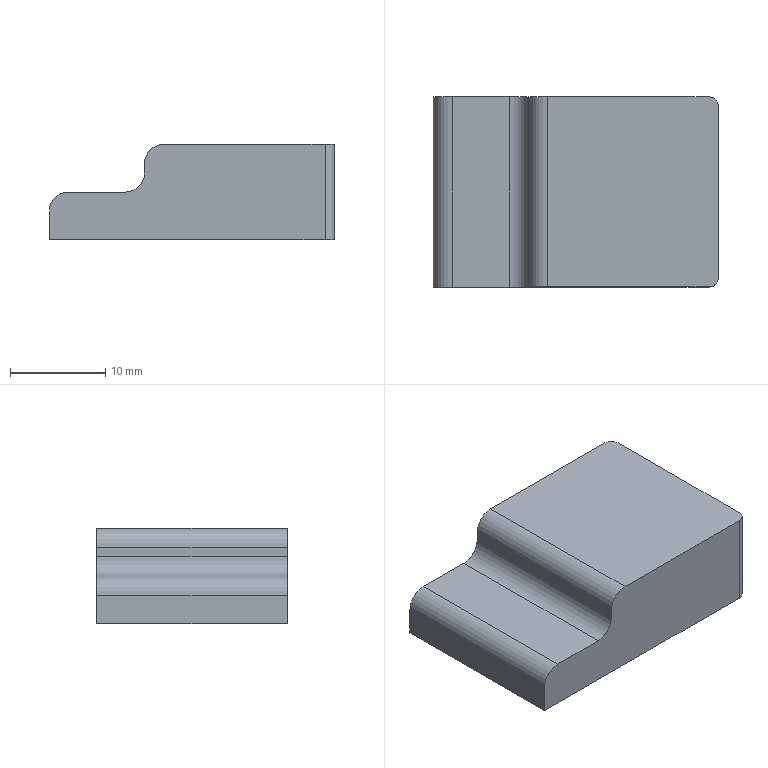Part | STEP file | Tube feed_id202_x_t | 1 solid | 13 faces | box 30 x 20 x 10 mm | volume 4979 mm3 | plane 8 | cylinder 5 | commonest cylinder face diameters 4 x3 2 x2
STEP:
#1=CARTESIAN_POINT('',(0.,0.,0.));
#2=DIRECTION('',(0.,0.,1.));
#3=DIRECTION('',(1.,0.,0.));
#4=AXIS2_PLACEMENT_3D('',#1,#2,#3);
#5=CARTESIAN_POINT('',(16.,401.936,-21.));
#6=VERTEX_POINT('',#5);
#7=CARTESIAN_POINT('',(16.,401.936,-18.));
#8=VERTEX_POINT('',#7);
#9=CARTESIAN_POINT('',(16.,401.936,-26.));
#10=DIRECTION('',(0.,0.,1.));
#11=VECTOR('',#10,1.);
#12=LINE('',#9,#11);
#13=CARTESIAN_POINT('',(16.,418.127,-26.));
#14=DIRECTION('',(-1.,0.,0.));
#15=DIRECTION('',(0.,0.,1.));
#16=AXIS2_PLACEMENT_3D('',#13,#14,#15);
#17=PLANE('',#16);
#18=CARTESIAN_POINT('',(0.,-16.192));
#19=DIRECTION('',(1.,0.));
#20=VECTOR('',#19,1.);
#21=LINE('',#18,#20);
#22=(GEOMETRIC_REPRESENTATION_CONTEXT(2)PARAMETRIC_REPRESENTATION_CONTEXT()REPRESENTATION_CONTEXT('',''));
#23=DEFINITIONAL_REPRESENTATION('',(#21),#22);
#24=PCURVE('',#17,#23);
#25=CARTESIAN_POINT('',(24.,401.936,-28.));
#26=DIRECTION('',(0.,1.,0.));
#27=DIRECTION('',(0.,0.,1.));
#28=AXIS2_PLACEMENT_3D('',#25,#26,#27);
#29=PLANE('',#28);
#30=CARTESIAN_POINT('',(2.,-8.));
#31=DIRECTION('',(1.,0.));
#32=VECTOR('',#31,1.);
#33=LINE('',#30,#32);
#34=(GEOMETRIC_REPRESENTATION_CONTEXT(2)PARAMETRIC_REPRESENTATION_CONTEXT()REPRESENTATION_CONTEXT('',''));
#35=DEFINITIONAL_REPRESENTATION('',(#33),#34);
#36=PCURVE('',#29,#35);
#37=SURFACE_CURVE('',#12,(#24,#36),.PCURVE_S1.);
#38=EDGE_CURVE('',#6,#8,#37,.T.);
#39=ORIENTED_EDGE('',*,*,#38,.T.);
#40=CARTESIAN_POINT('',(16.,421.936,-18.));
#41=VERTEX_POINT('',#40);
#42=CARTESIAN_POINT('',(16.,421.936,-18.));
#43=DIRECTION('',(0.,1.,0.));
#44=VECTOR('',#43,1.);
#45=LINE('',#42,#44);
#46=CARTESIAN_POINT('',(8.,3.808));
#47=DIRECTION('',(0.,1.));
#48=VECTOR('',#47,1.);
#49=LINE('',#46,#48);
#50=(GEOMETRIC_REPRESENTATION_CONTEXT(2)PARAMETRIC_REPRESENTATION_CONTEXT()REPRESENTATION_CONTEXT('',''));
#51=DEFINITIONAL_REPRESENTATION('',(#49),#50);
#52=PCURVE('',#17,#51);
#53=CARTESIAN_POINT('',(18.,383.127,-18.));
#54=DIRECTION('',(0.,1.,0.));
#55=DIRECTION('',(0.,0.,1.));
#56=AXIS2_PLACEMENT_3D('',#53,#54,#55);
#57=CYLINDRICAL_SURFACE('',#56,2.);
#58=CARTESIAN_POINT('',(4.712,38.808));
#59=DIRECTION('',(0.,1.));
#60=VECTOR('',#59,1.);
#61=LINE('',#58,#60);
#62=(GEOMETRIC_REPRESENTATION_CONTEXT(2)PARAMETRIC_REPRESENTATION_CONTEXT()REPRESENTATION_CONTEXT('',''));
#63=DEFINITIONAL_REPRESENTATION('',(#61),#62);
#64=PCURVE('',#57,#63);
#65=SURFACE_CURVE('',#45,(#52,#64),.PCURVE_S1.);
#66=EDGE_CURVE('',#8,#41,#65,.T.);
#67=ORIENTED_EDGE('',*,*,#66,.T.);
#68=CARTESIAN_POINT('',(16.,421.936,-21.));
#69=VERTEX_POINT('',#68);
#70=CARTESIAN_POINT('',(16.,421.936,-5.));
#71=DIRECTION('',(0.,0.,1.));
#72=VECTOR('',#71,1.);
#73=LINE('',#70,#72);
#74=CARTESIAN_POINT('',(21.,3.808));
#75=DIRECTION('',(1.,0.));
#76=VECTOR('',#75,1.);
#77=LINE('',#74,#76);
#78=(GEOMETRIC_REPRESENTATION_CONTEXT(2)PARAMETRIC_REPRESENTATION_CONTEXT()REPRESENTATION_CONTEXT('',''));
#79=DEFINITIONAL_REPRESENTATION('',(#77),#78);
#80=PCURVE('',#17,#79);
#81=CARTESIAN_POINT('',(0.,421.936,-5.));
#82=DIRECTION('',(0.,1.,0.));
#83=DIRECTION('',(0.,0.,1.));
#84=AXIS2_PLACEMENT_3D('',#81,#82,#83);
#85=PLANE('',#84);
#86=CARTESIAN_POINT('',(0.,16.));
#87=DIRECTION('',(1.,0.));
#88=VECTOR('',#87,1.);
#89=LINE('',#86,#88);
#90=(GEOMETRIC_REPRESENTATION_CONTEXT(2)PARAMETRIC_REPRESENTATION_CONTEXT()REPRESENTATION_CONTEXT('',''));
#91=DEFINITIONAL_REPRESENTATION('',(#89),#90);
#92=PCURVE('',#85,#91);
#93=SURFACE_CURVE('',#73,(#80,#92),.PCURVE_S1.);
#94=EDGE_CURVE('',#69,#41,#93,.T.);
#95=ORIENTED_EDGE('',*,*,#94,.F.);
#96=CARTESIAN_POINT('',(16.,0.,-21.));
#97=DIRECTION('',(0.,-1.,0.));
#98=VECTOR('',#97,1.);
#99=LINE('',#96,#98);
#100=CARTESIAN_POINT('',(5.,-418.127));
#101=DIRECTION('',(0.,-1.));
#102=VECTOR('',#101,1.);
#103=LINE('',#100,#102);
#104=(GEOMETRIC_REPRESENTATION_CONTEXT(2)PARAMETRIC_REPRESENTATION_CONTEXT()REPRESENTATION_CONTEXT('',''));
#105=DEFINITIONAL_REPRESENTATION('',(#103),#104);
#106=PCURVE('',#17,#105);
#107=CARTESIAN_POINT('',(0.,0.,-21.));
#108=DIRECTION('',(0.,0.,1.));
#109=DIRECTION('',(1.,0.,0.));
#110=AXIS2_PLACEMENT_3D('',#107,#108,#109);
#111=PLANE('',#110);
#112=CARTESIAN_POINT('',(16.,0.));
#113=DIRECTION('',(0.,-1.));
#114=VECTOR('',#113,1.);
#115=LINE('',#112,#114);
#116=(GEOMETRIC_REPRESENTATION_CONTEXT(2)PARAMETRIC_REPRESENTATION_CONTEXT()REPRESENTATION_CONTEXT('',''));
#117=DEFINITIONAL_REPRESENTATION('',(#115),#116);
#118=PCURVE('',#111,#117);
#119=SURFACE_CURVE('',#99,(#106,#118),.PCURVE_S1.);
#120=EDGE_CURVE('',#69,#6,#119,.T.);
#121=ORIENTED_EDGE('',*,*,#120,.T.);
#122=EDGE_LOOP('',(#39,#67,#95,#121));
#123=FACE_BOUND('',#122,.T.);
#124=ADVANCED_FACE('',(#123),#17,.T.);
#125=CARTESIAN_POINT('',(45.,401.936,-21.));
#126=VERTEX_POINT('',#125);
#127=CARTESIAN_POINT('',(0.,401.936,-21.));
#128=DIRECTION('',(1.,0.,0.));
#129=VECTOR('',#128,1.);
#130=LINE('',#127,#129);
#131=CARTESIAN_POINT('',(7.,-24.));
#132=DIRECTION('',(0.,1.));
#133=VECTOR('',#132,1.);
#134=LINE('',#131,#133);
#135=(GEOMETRIC_REPRESENTATION_CONTEXT(2)PARAMETRIC_REPRESENTATION_CONTEXT()REPRESENTATION_CONTEXT('',''));
#136=DEFINITIONAL_REPRESENTATION('',(#134),#135);
#137=PCURVE('',#29,#136);
#138=CARTESIAN_POINT('',(0.,401.936));
#139=DIRECTION('',(1.,0.));
#140=VECTOR('',#139,1.);
#141=LINE('',#138,#140);
#142=(GEOMETRIC_REPRESENTATION_CONTEXT(2)PARAMETRIC_REPRESENTATION_CONTEXT()REPRESENTATION_CONTEXT('',''));
#143=DEFINITIONAL_REPRESENTATION('',(#141),#142);
#144=PCURVE('',#111,#143);
#145=SURFACE_CURVE('',#130,(#137,#144),.PCURVE_S1.);
#146=EDGE_CURVE('',#6,#126,#145,.T.);
#147=ORIENTED_EDGE('',*,*,#146,.T.);
#148=CARTESIAN_POINT('',(45.,401.936,-11.));
#149=VERTEX_POINT('',#148);
#150=CARTESIAN_POINT('',(45.,401.936,-28.));
#151=DIRECTION('',(0.,0.,1.));
#152=VECTOR('',#151,1.);
#153=LINE('',#150,#152);
#154=CARTESIAN_POINT('',(0.,21.));
#155=DIRECTION('',(1.,0.));
#156=VECTOR('',#155,1.);
#157=LINE('',#154,#156);
#158=(GEOMETRIC_REPRESENTATION_CONTEXT(2)PARAMETRIC_REPRESENTATION_CONTEXT()REPRESENTATION_CONTEXT('',''));
#159=DEFINITIONAL_REPRESENTATION('',(#157),#158);
#160=PCURVE('',#29,#159);
#161=CARTESIAN_POINT('',(45.,402.936,-28.));
#162=DIRECTION('',(0.,0.,-1.));
#163=DIRECTION('',(0.,1.,0.));
#164=AXIS2_PLACEMENT_3D('',#161,#162,#163);
#165=CYLINDRICAL_SURFACE('',#164,1.);
#166=CARTESIAN_POINT('',(3.142,0.));
#167=DIRECTION('',(0.,-1.));
#168=VECTOR('',#167,1.);
#169=LINE('',#166,#168);
#170=(GEOMETRIC_REPRESENTATION_CONTEXT(2)PARAMETRIC_REPRESENTATION_CONTEXT()REPRESENTATION_CONTEXT('',''));
#171=DEFINITIONAL_REPRESENTATION('',(#169),#170);
#172=PCURVE('',#165,#171);
#173=SURFACE_CURVE('',#153,(#160,#172),.PCURVE_S1.);
#174=EDGE_CURVE('',#126,#149,#173,.T.);
#175=ORIENTED_EDGE('',*,*,#174,.T.);
#176=CARTESIAN_POINT('',(28.,401.936,-11.));
#177=VERTEX_POINT('',#176);
#178=CARTESIAN_POINT('',(-249.,401.936,-11.));
#179=DIRECTION('',(1.,0.,0.));
#180=VECTOR('',#179,1.);
#181=LINE('',#178,#180);
#182=CARTESIAN_POINT('',(17.,-273.));
#183=DIRECTION('',(0.,1.));
#184=VECTOR('',#183,1.);
#185=LINE('',#182,#184);
#186=(GEOMETRIC_REPRESENTATION_CONTEXT(2)PARAMETRIC_REPRESENTATION_CONTEXT()REPRESENTATION_CONTEXT('',''));
#187=DEFINITIONAL_REPRESENTATION('',(#185),#186);
#188=PCURVE('',#29,#187);
#189=CARTESIAN_POINT('',(-249.,30.286,-11.));
#190=DIRECTION('',(0.,0.,1.));
#191=DIRECTION('',(0.,-1.,0.));
#192=AXIS2_PLACEMENT_3D('',#189,#190,#191);
#193=PLANE('',#192);
#194=CARTESIAN_POINT('',(-371.65,0.));
#195=DIRECTION('',(0.,1.));
#196=VECTOR('',#195,1.);
#197=LINE('',#194,#196);
#198=(GEOMETRIC_REPRESENTATION_CONTEXT(2)PARAMETRIC_REPRESENTATION_CONTEXT()REPRESENTATION_CONTEXT('',''));
#199=DEFINITIONAL_REPRESENTATION('',(#197),#198);
#200=PCURVE('',#193,#199);
#201=SURFACE_CURVE('',#181,(#188,#200),.PCURVE_S1.);
#202=EDGE_CURVE('',#177,#149,#201,.T.);
#203=ORIENTED_EDGE('',*,*,#202,.F.);
#204=CARTESIAN_POINT('',(26.,401.936,-13.));
#205=VERTEX_POINT('',#204);
#206=CARTESIAN_POINT('',(28.,401.936,-13.));
#207=DIRECTION('',(0.,-1.,0.));
#208=DIRECTION('',(0.,0.,1.));
#209=AXIS2_PLACEMENT_3D('',#206,#207,#208);
#210=CIRCLE('',#209,2.);
#211=CARTESIAN_POINT('',(17.,4.));
#212=CARTESIAN_POINT('',(17.,0.5359));
#213=CARTESIAN_POINT('',(14.,2.268));
#214=CARTESIAN_POINT('',(11.,4.));
#215=CARTESIAN_POINT('',(14.,5.732));
#216=CARTESIAN_POINT('',(17.,7.464));
#217=CARTESIAN_POINT('',(17.,4.));
#218=(BOUNDED_CURVE()B_SPLINE_CURVE(2,(#211,#212,#213,#214,#215,#216,#217),.UNSPECIFIED.,.T.,.F.)B_SPLINE_CURVE_WITH_KNOTS((1,2,2,2,2,1),(-2.094,0.,2.094,4.189,6.283,8.378),.UNSPECIFIED.)CURVE()GEOMETRIC_REPRESENTATION_ITEM()RATIONAL_B_SPLINE_CURVE((1.,0.5,1.,0.5,1.,0.5,1.))REPRESENTATION_ITEM(''));
#219=(GEOMETRIC_REPRESENTATION_CONTEXT(2)PARAMETRIC_REPRESENTATION_CONTEXT()REPRESENTATION_CONTEXT('',''));
#220=DEFINITIONAL_REPRESENTATION('',(#218),#219);
#221=PCURVE('',#29,#220);
#222=CARTESIAN_POINT('',(28.,383.127,-13.));
#223=DIRECTION('',(0.,-1.,0.));
#224=DIRECTION('',(0.,0.,-1.));
#225=AXIS2_PLACEMENT_3D('',#222,#223,#224);
#226=CYLINDRICAL_SURFACE('',#225,2.);
#227=CARTESIAN_POINT('',(3.142,-18.808));
#228=DIRECTION('',(1.,0.));
#229=VECTOR('',#228,1.);
#230=LINE('',#227,#229);
#231=(GEOMETRIC_REPRESENTATION_CONTEXT(2)PARAMETRIC_REPRESENTATION_CONTEXT()REPRESENTATION_CONTEXT('',''));
#232=DEFINITIONAL_REPRESENTATION('',(#230),#231);
#233=PCURVE('',#226,#232);
#234=SURFACE_CURVE('',#210,(#221,#233),.PCURVE_S1.);
#235=EDGE_CURVE('',#177,#205,#234,.T.);
#236=ORIENTED_EDGE('',*,*,#235,.T.);
#237=CARTESIAN_POINT('',(26.,401.936,-14.));
#238=VERTEX_POINT('',#237);
#239=CARTESIAN_POINT('',(26.,401.936,-28.));
#240=DIRECTION('',(0.,0.,1.));
#241=VECTOR('',#240,1.);
#242=LINE('',#239,#241);
#243=CARTESIAN_POINT('',(0.,2.));
#244=DIRECTION('',(1.,0.));
#245=VECTOR('',#244,1.);
#246=LINE('',#243,#245);
#247=(GEOMETRIC_REPRESENTATION_CONTEXT(2)PARAMETRIC_REPRESENTATION_CONTEXT()REPRESENTATION_CONTEXT('',''));
#248=DEFINITIONAL_REPRESENTATION('',(#246),#247);
#249=PCURVE('',#29,#248);
#250=CARTESIAN_POINT('',(26.,383.127,-7.5));
#251=DIRECTION('',(1.,0.,0.));
#252=DIRECTION('',(0.,0.,-1.));
#253=AXIS2_PLACEMENT_3D('',#250,#251,#252);
#254=PLANE('',#253);
#255=CARTESIAN_POINT('',(20.5,18.808));
#256=DIRECTION('',(-1.,0.));
#257=VECTOR('',#256,1.);
#258=LINE('',#255,#257);
#259=(GEOMETRIC_REPRESENTATION_CONTEXT(2)PARAMETRIC_REPRESENTATION_CONTEXT()REPRESENTATION_CONTEXT('',''));
#260=DEFINITIONAL_REPRESENTATION('',(#258),#259);
#261=PCURVE('',#254,#260);
#262=SURFACE_CURVE('',#242,(#249,#261),.PCURVE_S1.);
#263=EDGE_CURVE('',#238,#205,#262,.T.);
#264=ORIENTED_EDGE('',*,*,#263,.F.);
#265=CARTESIAN_POINT('',(24.,401.936,-16.));
#266=VERTEX_POINT('',#265);
#267=CARTESIAN_POINT('',(24.,401.936,-14.));
#268=DIRECTION('',(0.,1.,0.));
#269=DIRECTION('',(0.,0.,1.));
#270=AXIS2_PLACEMENT_3D('',#267,#268,#269);
#271=CIRCLE('',#270,2.);
#272=CARTESIAN_POINT('',(14.,0.));
#273=DIRECTION('',(1.,0.));
#274=AXIS2_PLACEMENT_2D('',#272,#273);
#275=CIRCLE('',#274,2.);
#276=(GEOMETRIC_REPRESENTATION_CONTEXT(2)PARAMETRIC_REPRESENTATION_CONTEXT()REPRESENTATION_CONTEXT('',''));
#277=DEFINITIONAL_REPRESENTATION('',(#275),#276);
#278=PCURVE('',#29,#277);
#279=CARTESIAN_POINT('',(24.,383.127,-14.));
#280=DIRECTION('',(0.,1.,0.));
#281=DIRECTION('',(0.,0.,1.));
#282=AXIS2_PLACEMENT_3D('',#279,#280,#281);
#283=CYLINDRICAL_SURFACE('',#282,2.);
#284=CARTESIAN_POINT('',(0.,18.808));
#285=DIRECTION('',(1.,0.));
#286=VECTOR('',#285,1.);
#287=LINE('',#284,#286);
#288=(GEOMETRIC_REPRESENTATION_CONTEXT(2)PARAMETRIC_REPRESENTATION_CONTEXT()REPRESENTATION_CONTEXT('',''));
#289=DEFINITIONAL_REPRESENTATION('',(#287),#288);
#290=PCURVE('',#283,#289);
#291=SURFACE_CURVE('',#271,(#278,#290),.PCURVE_S1.);
#292=EDGE_CURVE('',#238,#266,#291,.T.);
#293=ORIENTED_EDGE('',*,*,#292,.T.);
#294=CARTESIAN_POINT('',(18.,401.936,-16.));
#295=VERTEX_POINT('',#294);
#296=CARTESIAN_POINT('',(24.,401.936,-16.));
#297=DIRECTION('',(1.,0.,0.));
#298=VECTOR('',#297,1.);
#299=LINE('',#296,#298);
#300=CARTESIAN_POINT('',(12.,0.));
#301=DIRECTION('',(0.,1.));
#302=VECTOR('',#301,1.);
#303=LINE('',#300,#302);
#304=(GEOMETRIC_REPRESENTATION_CONTEXT(2)PARAMETRIC_REPRESENTATION_CONTEXT()REPRESENTATION_CONTEXT('',''));
#305=DEFINITIONAL_REPRESENTATION('',(#303),#304);
#306=PCURVE('',#29,#305);
#307=CARTESIAN_POINT('',(26.,383.127,-16.));
#308=DIRECTION('',(0.,0.,-1.));
#309=DIRECTION('',(-1.,0.,0.));
#310=AXIS2_PLACEMENT_3D('',#307,#308,#309);
#311=PLANE('',#310);
#312=CARTESIAN_POINT('',(2.,18.808));
#313=DIRECTION('',(-1.,0.));
#314=VECTOR('',#313,1.);
#315=LINE('',#312,#314);
#316=(GEOMETRIC_REPRESENTATION_CONTEXT(2)PARAMETRIC_REPRESENTATION_CONTEXT()REPRESENTATION_CONTEXT('',''));
#317=DEFINITIONAL_REPRESENTATION('',(#315),#316);
#318=PCURVE('',#311,#317);
#319=SURFACE_CURVE('',#299,(#306,#318),.PCURVE_S1.);
#320=EDGE_CURVE('',#295,#266,#319,.T.);
#321=ORIENTED_EDGE('',*,*,#320,.F.);
#322=CARTESIAN_POINT('',(18.,401.936,-18.));
#323=DIRECTION('',(0.,-1.,0.));
#324=DIRECTION('',(0.,0.,1.));
#325=AXIS2_PLACEMENT_3D('',#322,#323,#324);
#326=CIRCLE('',#325,2.);
#327=CARTESIAN_POINT('',(12.,-6.));
#328=CARTESIAN_POINT('',(12.,-9.464));
#329=CARTESIAN_POINT('',(9.,-7.732));
#330=CARTESIAN_POINT('',(6.,-6.));
#331=CARTESIAN_POINT('',(9.,-4.268));
#332=CARTESIAN_POINT('',(12.,-2.536));
#333=CARTESIAN_POINT('',(12.,-6.));
#334=(BOUNDED_CURVE()B_SPLINE_CURVE(2,(#327,#328,#329,#330,#331,#332,#333),.UNSPECIFIED.,.T.,.F.)B_SPLINE_CURVE_WITH_KNOTS((1,2,2,2,2,1),(-2.094,0.,2.094,4.189,6.283,8.378),.UNSPECIFIED.)CURVE()GEOMETRIC_REPRESENTATION_ITEM()RATIONAL_B_SPLINE_CURVE((1.,0.5,1.,0.5,1.,0.5,1.))REPRESENTATION_ITEM(''));
#335=(GEOMETRIC_REPRESENTATION_CONTEXT(2)PARAMETRIC_REPRESENTATION_CONTEXT()REPRESENTATION_CONTEXT('',''));
#336=DEFINITIONAL_REPRESENTATION('',(#334),#335);
#337=PCURVE('',#29,#336);
#338=CARTESIAN_POINT('',(6.283,18.808));
#339=DIRECTION('',(-1.,0.));
#340=VECTOR('',#339,1.);
#341=LINE('',#338,#340);
#342=(GEOMETRIC_REPRESENTATION_CONTEXT(2)PARAMETRIC_REPRESENTATION_CONTEXT()REPRESENTATION_CONTEXT('',''));
#343=DEFINITIONAL_REPRESENTATION('',(#341),#342);
#344=PCURVE('',#57,#343);
#345=SURFACE_CURVE('',#326,(#337,#344),.PCURVE_S1.);
#346=EDGE_CURVE('',#295,#8,#345,.T.);
#347=ORIENTED_EDGE('',*,*,#346,.T.);
#348=ORIENTED_EDGE('',*,*,#38,.F.);
#349=EDGE_LOOP('',(#147,#175,#203,#236,#264,#293,#321,#347,#348));
#350=FACE_BOUND('',#349,.T.);
#351=ADVANCED_FACE('',(#350),#29,.F.);
#352=CARTESIAN_POINT('',(46.,402.936,-21.));
#353=VERTEX_POINT('',#352);
#354=CARTESIAN_POINT('',(46.,420.936,-21.));
#355=VERTEX_POINT('',#354);
#356=CARTESIAN_POINT('',(46.,0.,-21.));
#357=DIRECTION('',(0.,1.,0.));
#358=VECTOR('',#357,1.);
#359=LINE('',#356,#358);
#360=CARTESIAN_POINT('',(46.,361.936,-26.));
#361=DIRECTION('',(1.,0.,0.));
#362=DIRECTION('',(0.,0.,-1.));
#363=AXIS2_PLACEMENT_3D('',#360,#361,#362);
#364=PLANE('',#363);
#365=CARTESIAN_POINT('',(-5.,-361.936));
#366=DIRECTION('',(0.,1.));
#367=VECTOR('',#366,1.);
#368=LINE('',#365,#367);
#369=(GEOMETRIC_REPRESENTATION_CONTEXT(2)PARAMETRIC_REPRESENTATION_CONTEXT()REPRESENTATION_CONTEXT('',''));
#370=DEFINITIONAL_REPRESENTATION('',(#368),#369);
#371=PCURVE('',#364,#370);
#372=CARTESIAN_POINT('',(46.,0.));
#373=DIRECTION('',(0.,1.));
#374=VECTOR('',#373,1.);
#375=LINE('',#372,#374);
#376=(GEOMETRIC_REPRESENTATION_CONTEXT(2)PARAMETRIC_REPRESENTATION_CONTEXT()REPRESENTATION_CONTEXT('',''));
#377=DEFINITIONAL_REPRESENTATION('',(#375),#376);
#378=PCURVE('',#111,#377);
#379=SURFACE_CURVE('',#359,(#371,#378),.PCURVE_S1.);
#380=EDGE_CURVE('',#353,#355,#379,.T.);
#381=ORIENTED_EDGE('',*,*,#380,.T.);
#382=CARTESIAN_POINT('',(46.,420.936,-11.));
#383=VERTEX_POINT('',#382);
#384=CARTESIAN_POINT('',(46.,420.936,-26.));
#385=DIRECTION('',(0.,0.,1.));
#386=VECTOR('',#385,1.);
#387=LINE('',#384,#386);
#388=CARTESIAN_POINT('',(0.,59.));
#389=DIRECTION('',(-1.,0.));
#390=VECTOR('',#389,1.);
#391=LINE('',#388,#390);
#392=(GEOMETRIC_REPRESENTATION_CONTEXT(2)PARAMETRIC_REPRESENTATION_CONTEXT()REPRESENTATION_CONTEXT('',''));
#393=DEFINITIONAL_REPRESENTATION('',(#391),#392);
#394=PCURVE('',#364,#393);
#395=CARTESIAN_POINT('',(45.,420.936,-26.));
#396=DIRECTION('',(0.,0.,1.));
#397=DIRECTION('',(1.,0.,0.));
#398=AXIS2_PLACEMENT_3D('',#395,#396,#397);
#399=CYLINDRICAL_SURFACE('',#398,1.);
#400=CARTESIAN_POINT('',(0.,0.));
#401=DIRECTION('',(0.,1.));
#402=VECTOR('',#401,1.);
#403=LINE('',#400,#402);
#404=(GEOMETRIC_REPRESENTATION_CONTEXT(2)PARAMETRIC_REPRESENTATION_CONTEXT()REPRESENTATION_CONTEXT('',''));
#405=DEFINITIONAL_REPRESENTATION('',(#403),#404);
#406=PCURVE('',#399,#405);
#407=SURFACE_CURVE('',#387,(#394,#406),.PCURVE_S1.);
#408=EDGE_CURVE('',#355,#383,#407,.T.);
#409=ORIENTED_EDGE('',*,*,#408,.T.);
#410=CARTESIAN_POINT('',(46.,402.936,-11.));
#411=VERTEX_POINT('',#410);
#412=CARTESIAN_POINT('',(46.,30.286,-11.));
#413=DIRECTION('',(0.,1.,0.));
#414=VECTOR('',#413,1.);
#415=LINE('',#412,#414);
#416=CARTESIAN_POINT('',(-15.,-331.65));
#417=DIRECTION('',(0.,1.));
#418=VECTOR('',#417,1.);
#419=LINE('',#416,#418);
#420=(GEOMETRIC_REPRESENTATION_CONTEXT(2)PARAMETRIC_REPRESENTATION_CONTEXT()REPRESENTATION_CONTEXT('',''));
#421=DEFINITIONAL_REPRESENTATION('',(#419),#420);
#422=PCURVE('',#364,#421);
#423=CARTESIAN_POINT('',(0.,295.));
#424=DIRECTION('',(-1.,0.));
#425=VECTOR('',#424,1.);
#426=LINE('',#423,#425);
#427=(GEOMETRIC_REPRESENTATION_CONTEXT(2)PARAMETRIC_REPRESENTATION_CONTEXT()REPRESENTATION_CONTEXT('',''));
#428=DEFINITIONAL_REPRESENTATION('',(#426),#427);
#429=PCURVE('',#193,#428);
#430=SURFACE_CURVE('',#415,(#422,#429),.PCURVE_S1.);
#431=EDGE_CURVE('',#411,#383,#430,.T.);
#432=ORIENTED_EDGE('',*,*,#431,.F.);
#433=CARTESIAN_POINT('',(46.,402.936,-26.));
#434=DIRECTION('',(0.,0.,-1.));
#435=VECTOR('',#434,1.);
#436=LINE('',#433,#435);
#437=CARTESIAN_POINT('',(0.,41.));
#438=DIRECTION('',(1.,0.));
#439=VECTOR('',#438,1.);
#440=LINE('',#437,#439);
#441=(GEOMETRIC_REPRESENTATION_CONTEXT(2)PARAMETRIC_REPRESENTATION_CONTEXT()REPRESENTATION_CONTEXT('',''));
#442=DEFINITIONAL_REPRESENTATION('',(#440),#441);
#443=PCURVE('',#364,#442);
#444=CARTESIAN_POINT('',(1.571,-2.));
#445=DIRECTION('',(0.,1.));
#446=VECTOR('',#445,1.);
#447=LINE('',#444,#446);
#448=(GEOMETRIC_REPRESENTATION_CONTEXT(2)PARAMETRIC_REPRESENTATION_CONTEXT()REPRESENTATION_CONTEXT('',''));
#449=DEFINITIONAL_REPRESENTATION('',(#447),#448);
#450=PCURVE('',#165,#449);
#451=SURFACE_CURVE('',#436,(#443,#450),.PCURVE_S1.);
#452=EDGE_CURVE('',#411,#353,#451,.T.);
#453=ORIENTED_EDGE('',*,*,#452,.T.);
#454=EDGE_LOOP('',(#381,#409,#432,#453));
#455=FACE_BOUND('',#454,.T.);
#456=ADVANCED_FACE('',(#455),#364,.T.);
#457=CARTESIAN_POINT('',(45.,421.936,-11.));
#458=VERTEX_POINT('',#457);
#459=CARTESIAN_POINT('',(28.,421.936,-11.));
#460=VERTEX_POINT('',#459);
#461=CARTESIAN_POINT('',(-249.,421.936,-11.));
#462=DIRECTION('',(-1.,0.,0.));
#463=VECTOR('',#462,1.);
#464=LINE('',#461,#463);
#465=CARTESIAN_POINT('',(-6.,-249.));
#466=DIRECTION('',(0.,-1.));
#467=VECTOR('',#466,1.);
#468=LINE('',#465,#467);
#469=(GEOMETRIC_REPRESENTATION_CONTEXT(2)PARAMETRIC_REPRESENTATION_CONTEXT()REPRESENTATION_CONTEXT('',''));
#470=DEFINITIONAL_REPRESENTATION('',(#468),#469);
#471=PCURVE('',#85,#470);
#472=CARTESIAN_POINT('',(-391.65,0.));
#473=DIRECTION('',(0.,-1.));
#474=VECTOR('',#473,1.);
#475=LINE('',#472,#474);
#476=(GEOMETRIC_REPRESENTATION_CONTEXT(2)PARAMETRIC_REPRESENTATION_CONTEXT()REPRESENTATION_CONTEXT('',''));
#477=DEFINITIONAL_REPRESENTATION('',(#475),#476);
#478=PCURVE('',#193,#477);
#479=SURFACE_CURVE('',#464,(#471,#478),.PCURVE_S1.);
#480=EDGE_CURVE('',#458,#460,#479,.T.);
#481=ORIENTED_EDGE('',*,*,#480,.F.);
#482=CARTESIAN_POINT('',(45.,421.936,-21.));
#483=VERTEX_POINT('',#482);
#484=CARTESIAN_POINT('',(45.,421.936,-5.));
#485=DIRECTION('',(0.,0.,-1.));
#486=VECTOR('',#485,1.);
#487=LINE('',#484,#486);
#488=CARTESIAN_POINT('',(0.,45.));
#489=DIRECTION('',(-1.,0.));
#490=VECTOR('',#489,1.);
#491=LINE('',#488,#490);
#492=(GEOMETRIC_REPRESENTATION_CONTEXT(2)PARAMETRIC_REPRESENTATION_CONTEXT()REPRESENTATION_CONTEXT('',''));
#493=DEFINITIONAL_REPRESENTATION('',(#491),#492);
#494=PCURVE('',#85,#493);
#495=CARTESIAN_POINT('',(1.571,21.));
#496=DIRECTION('',(0.,-1.));
#497=VECTOR('',#496,1.);
#498=LINE('',#495,#497);
#499=(GEOMETRIC_REPRESENTATION_CONTEXT(2)PARAMETRIC_REPRESENTATION_CONTEXT()REPRESENTATION_CONTEXT('',''));
#500=DEFINITIONAL_REPRESENTATION('',(#498),#499);
#501=PCURVE('',#399,#500);
#502=SURFACE_CURVE('',#487,(#494,#501),.PCURVE_S1.);
#503=EDGE_CURVE('',#458,#483,#502,.T.);
#504=ORIENTED_EDGE('',*,*,#503,.T.);
#505=CARTESIAN_POINT('',(0.,421.936,-21.));
#506=DIRECTION('',(-1.,0.,0.));
#507=VECTOR('',#506,1.);
#508=LINE('',#505,#507);
#509=CARTESIAN_POINT('',(-16.,0.));
#510=DIRECTION('',(0.,-1.));
#511=VECTOR('',#510,1.);
#512=LINE('',#509,#511);
#513=(GEOMETRIC_REPRESENTATION_CONTEXT(2)PARAMETRIC_REPRESENTATION_CONTEXT()REPRESENTATION_CONTEXT('',''));
#514=DEFINITIONAL_REPRESENTATION('',(#512),#513);
#515=PCURVE('',#85,#514);
#516=CARTESIAN_POINT('',(0.,421.936));
#517=DIRECTION('',(-1.,0.));
#518=VECTOR('',#517,1.);
#519=LINE('',#516,#518);
#520=(GEOMETRIC_REPRESENTATION_CONTEXT(2)PARAMETRIC_REPRESENTATION_CONTEXT()REPRESENTATION_CONTEXT('',''));
#521=DEFINITIONAL_REPRESENTATION('',(#519),#520);
#522=PCURVE('',#111,#521);
#523=SURFACE_CURVE('',#508,(#515,#522),.PCURVE_S1.);
#524=EDGE_CURVE('',#483,#69,#523,.T.);
#525=ORIENTED_EDGE('',*,*,#524,.T.);
#526=ORIENTED_EDGE('',*,*,#94,.T.);
#527=CARTESIAN_POINT('',(18.,421.936,-16.));
#528=VERTEX_POINT('',#527);
#529=CARTESIAN_POINT('',(18.,421.936,-18.));
#530=DIRECTION('',(0.,1.,0.));
#531=DIRECTION('',(0.,0.,1.));
#532=AXIS2_PLACEMENT_3D('',#529,#530,#531);
#533=CIRCLE('',#532,2.);
#534=CARTESIAN_POINT('',(-13.,18.));
#535=DIRECTION('',(1.,0.));
#536=AXIS2_PLACEMENT_2D('',#534,#535);
#537=CIRCLE('',#536,2.);
#538=(GEOMETRIC_REPRESENTATION_CONTEXT(2)PARAMETRIC_REPRESENTATION_CONTEXT()REPRESENTATION_CONTEXT('',''));
#539=DEFINITIONAL_REPRESENTATION('',(#537),#538);
#540=PCURVE('',#85,#539);
#541=CARTESIAN_POINT('',(0.,38.808));
#542=DIRECTION('',(1.,0.));
#543=VECTOR('',#542,1.);
#544=LINE('',#541,#543);
#545=(GEOMETRIC_REPRESENTATION_CONTEXT(2)PARAMETRIC_REPRESENTATION_CONTEXT()REPRESENTATION_CONTEXT('',''));
#546=DEFINITIONAL_REPRESENTATION('',(#544),#545);
#547=PCURVE('',#57,#546);
#548=SURFACE_CURVE('',#533,(#540,#547),.PCURVE_S1.);
#549=EDGE_CURVE('',#41,#528,#548,.T.);
#550=ORIENTED_EDGE('',*,*,#549,.T.);
#551=CARTESIAN_POINT('',(24.,421.936,-16.));
#552=VERTEX_POINT('',#551);
#553=CARTESIAN_POINT('',(0.,421.936,-16.));
#554=DIRECTION('',(-1.,0.,0.));
#555=VECTOR('',#554,1.);
#556=LINE('',#553,#555);
#557=CARTESIAN_POINT('',(-11.,0.));
#558=DIRECTION('',(0.,-1.));
#559=VECTOR('',#558,1.);
#560=LINE('',#557,#559);
#561=(GEOMETRIC_REPRESENTATION_CONTEXT(2)PARAMETRIC_REPRESENTATION_CONTEXT()REPRESENTATION_CONTEXT('',''));
#562=DEFINITIONAL_REPRESENTATION('',(#560),#561);
#563=PCURVE('',#85,#562);
#564=CARTESIAN_POINT('',(26.,38.808));
#565=DIRECTION('',(1.,0.));
#566=VECTOR('',#565,1.);
#567=LINE('',#564,#566);
#568=(GEOMETRIC_REPRESENTATION_CONTEXT(2)PARAMETRIC_REPRESENTATION_CONTEXT()REPRESENTATION_CONTEXT('',''));
#569=DEFINITIONAL_REPRESENTATION('',(#567),#568);
#570=PCURVE('',#311,#569);
#571=SURFACE_CURVE('',#556,(#563,#570),.PCURVE_S1.);
#572=EDGE_CURVE('',#552,#528,#571,.T.);
#573=ORIENTED_EDGE('',*,*,#572,.F.);
#574=CARTESIAN_POINT('',(26.,421.936,-14.));
#575=VERTEX_POINT('',#574);
#576=CARTESIAN_POINT('',(24.,421.936,-14.));
#577=DIRECTION('',(0.,-1.,0.));
#578=DIRECTION('',(0.,0.,1.));
#579=AXIS2_PLACEMENT_3D('',#576,#577,#578);
#580=CIRCLE('',#579,2.);
#581=CARTESIAN_POINT('',(-7.,24.));
#582=CARTESIAN_POINT('',(-7.,20.536));
#583=CARTESIAN_POINT('',(-10.,22.268));
#584=CARTESIAN_POINT('',(-13.,24.));
#585=CARTESIAN_POINT('',(-10.,25.732));
#586=CARTESIAN_POINT('',(-7.,27.464));
#587=CARTESIAN_POINT('',(-7.,24.));
#588=(BOUNDED_CURVE()B_SPLINE_CURVE(2,(#581,#582,#583,#584,#585,#586,#587),.UNSPECIFIED.,.T.,.F.)B_SPLINE_CURVE_WITH_KNOTS((1,2,2,2,2,1),(-2.094,0.,2.094,4.189,6.283,8.378),.UNSPECIFIED.)CURVE()GEOMETRIC_REPRESENTATION_ITEM()RATIONAL_B_SPLINE_CURVE((1.,0.5,1.,0.5,1.,0.5,1.))REPRESENTATION_ITEM(''));
#589=(GEOMETRIC_REPRESENTATION_CONTEXT(2)PARAMETRIC_REPRESENTATION_CONTEXT()REPRESENTATION_CONTEXT('',''));
#590=DEFINITIONAL_REPRESENTATION('',(#588),#589);
#591=PCURVE('',#85,#590);
#592=CARTESIAN_POINT('',(6.283,38.808));
#593=DIRECTION('',(-1.,0.));
#594=VECTOR('',#593,1.);
#595=LINE('',#592,#594);
#596=(GEOMETRIC_REPRESENTATION_CONTEXT(2)PARAMETRIC_REPRESENTATION_CONTEXT()REPRESENTATION_CONTEXT('',''));
#597=DEFINITIONAL_REPRESENTATION('',(#595),#596);
#598=PCURVE('',#283,#597);
#599=SURFACE_CURVE('',#580,(#591,#598),.PCURVE_S1.);
#600=EDGE_CURVE('',#552,#575,#599,.T.);
#601=ORIENTED_EDGE('',*,*,#600,.T.);
#602=CARTESIAN_POINT('',(26.,421.936,-13.));
#603=VERTEX_POINT('',#602);
#604=CARTESIAN_POINT('',(26.,421.936,-5.));
#605=DIRECTION('',(0.,0.,-1.));
#606=VECTOR('',#605,1.);
#607=LINE('',#604,#606);
#608=CARTESIAN_POINT('',(0.,26.));
#609=DIRECTION('',(-1.,0.));
#610=VECTOR('',#609,1.);
#611=LINE('',#608,#610);
#612=(GEOMETRIC_REPRESENTATION_CONTEXT(2)PARAMETRIC_REPRESENTATION_CONTEXT()REPRESENTATION_CONTEXT('',''));
#613=DEFINITIONAL_REPRESENTATION('',(#611),#612);
#614=PCURVE('',#85,#613);
#615=CARTESIAN_POINT('',(-2.5,38.808));
#616=DIRECTION('',(1.,0.));
#617=VECTOR('',#616,1.);
#618=LINE('',#615,#617);
#619=(GEOMETRIC_REPRESENTATION_CONTEXT(2)PARAMETRIC_REPRESENTATION_CONTEXT()REPRESENTATION_CONTEXT('',''));
#620=DEFINITIONAL_REPRESENTATION('',(#618),#619);
#621=PCURVE('',#254,#620);
#622=SURFACE_CURVE('',#607,(#614,#621),.PCURVE_S1.);
#623=EDGE_CURVE('',#603,#575,#622,.T.);
#624=ORIENTED_EDGE('',*,*,#623,.F.);
#625=CARTESIAN_POINT('',(28.,421.936,-13.));
#626=DIRECTION('',(0.,1.,0.));
#627=DIRECTION('',(0.,0.,1.));
#628=AXIS2_PLACEMENT_3D('',#625,#626,#627);
#629=CIRCLE('',#628,2.);
#630=CARTESIAN_POINT('',(-8.,28.));
#631=DIRECTION('',(1.,0.));
#632=AXIS2_PLACEMENT_2D('',#630,#631);
#633=CIRCLE('',#632,2.);
#634=(GEOMETRIC_REPRESENTATION_CONTEXT(2)PARAMETRIC_REPRESENTATION_CONTEXT()REPRESENTATION_CONTEXT('',''));
#635=DEFINITIONAL_REPRESENTATION('',(#633),#634);
#636=PCURVE('',#85,#635);
#637=CARTESIAN_POINT('',(9.425,-38.808));
#638=DIRECTION('',(-1.,0.));
#639=VECTOR('',#638,1.);
#640=LINE('',#637,#639);
#641=(GEOMETRIC_REPRESENTATION_CONTEXT(2)PARAMETRIC_REPRESENTATION_CONTEXT()REPRESENTATION_CONTEXT('',''));
#642=DEFINITIONAL_REPRESENTATION('',(#640),#641);
#643=PCURVE('',#226,#642);
#644=SURFACE_CURVE('',#629,(#636,#643),.PCURVE_S1.);
#645=EDGE_CURVE('',#603,#460,#644,.T.);
#646=ORIENTED_EDGE('',*,*,#645,.T.);
#647=EDGE_LOOP('',(#481,#504,#525,#526,#550,#573,#601,#624,#646));
#648=FACE_BOUND('',#647,.T.);
#649=ADVANCED_FACE('',(#648),#85,.T.);
#650=ORIENTED_EDGE('',*,*,#524,.F.);
#651=CARTESIAN_POINT('',(45.,420.936,-21.));
#652=DIRECTION('',(0.,0.,-1.));
#653=DIRECTION('',(1.,0.,0.));
#654=AXIS2_PLACEMENT_3D('',#651,#652,#653);
#655=CIRCLE('',#654,1.);
#656=CARTESIAN_POINT('',(46.,420.936));
#657=CARTESIAN_POINT('',(46.,419.204));
#658=CARTESIAN_POINT('',(44.5,420.07));
#659=CARTESIAN_POINT('',(43.,420.936));
#660=CARTESIAN_POINT('',(44.5,421.802));
#661=CARTESIAN_POINT('',(46.,422.668));
#662=CARTESIAN_POINT('',(46.,420.936));
#663=(BOUNDED_CURVE()B_SPLINE_CURVE(2,(#656,#657,#658,#659,#660,#661,#662),.UNSPECIFIED.,.T.,.F.)B_SPLINE_CURVE_WITH_KNOTS((1,2,2,2,2,1),(-2.094,0.,2.094,4.189,6.283,8.378),.UNSPECIFIED.)CURVE()GEOMETRIC_REPRESENTATION_ITEM()RATIONAL_B_SPLINE_CURVE((1.,0.5,1.,0.5,1.,0.5,1.))REPRESENTATION_ITEM(''));
#664=(GEOMETRIC_REPRESENTATION_CONTEXT(2)PARAMETRIC_REPRESENTATION_CONTEXT()REPRESENTATION_CONTEXT('',''));
#665=DEFINITIONAL_REPRESENTATION('',(#663),#664);
#666=PCURVE('',#111,#665);
#667=CARTESIAN_POINT('',(6.283,5.));
#668=DIRECTION('',(-1.,0.));
#669=VECTOR('',#668,1.);
#670=LINE('',#667,#669);
#671=(GEOMETRIC_REPRESENTATION_CONTEXT(2)PARAMETRIC_REPRESENTATION_CONTEXT()REPRESENTATION_CONTEXT('',''));
#672=DEFINITIONAL_REPRESENTATION('',(#670),#671);
#673=PCURVE('',#399,#672);
#674=SURFACE_CURVE('',#655,(#666,#673),.PCURVE_S1.);
#675=EDGE_CURVE('',#483,#355,#674,.T.);
#676=ORIENTED_EDGE('',*,*,#675,.T.);
#677=ORIENTED_EDGE('',*,*,#380,.F.);
#678=CARTESIAN_POINT('',(45.,402.936,-21.));
#679=DIRECTION('',(0.,0.,-1.));
#680=DIRECTION('',(1.,0.,0.));
#681=AXIS2_PLACEMENT_3D('',#678,#679,#680);
#682=CIRCLE('',#681,1.);
#683=CARTESIAN_POINT('',(46.,402.936));
#684=CARTESIAN_POINT('',(46.,401.204));
#685=CARTESIAN_POINT('',(44.5,402.07));
#686=CARTESIAN_POINT('',(43.,402.936));
#687=CARTESIAN_POINT('',(44.5,403.802));
#688=CARTESIAN_POINT('',(46.,404.668));
#689=CARTESIAN_POINT('',(46.,402.936));
#690=(BOUNDED_CURVE()B_SPLINE_CURVE(2,(#683,#684,#685,#686,#687,#688,#689),.UNSPECIFIED.,.T.,.F.)B_SPLINE_CURVE_WITH_KNOTS((1,2,2,2,2,1),(-2.094,0.,2.094,4.189,6.283,8.378),.UNSPECIFIED.)CURVE()GEOMETRIC_REPRESENTATION_ITEM()RATIONAL_B_SPLINE_CURVE((1.,0.5,1.,0.5,1.,0.5,1.))REPRESENTATION_ITEM(''));
#691=(GEOMETRIC_REPRESENTATION_CONTEXT(2)PARAMETRIC_REPRESENTATION_CONTEXT()REPRESENTATION_CONTEXT('',''));
#692=DEFINITIONAL_REPRESENTATION('',(#690),#691);
#693=PCURVE('',#111,#692);
#694=CARTESIAN_POINT('',(1.571,-7.));
#695=DIRECTION('',(1.,0.));
#696=VECTOR('',#695,1.);
#697=LINE('',#694,#696);
#698=(GEOMETRIC_REPRESENTATION_CONTEXT(2)PARAMETRIC_REPRESENTATION_CONTEXT()REPRESENTATION_CONTEXT('',''));
#699=DEFINITIONAL_REPRESENTATION('',(#697),#698);
#700=PCURVE('',#165,#699);
#701=SURFACE_CURVE('',#682,(#693,#700),.PCURVE_S1.);
#702=EDGE_CURVE('',#353,#126,#701,.T.);
#703=ORIENTED_EDGE('',*,*,#702,.T.);
#704=ORIENTED_EDGE('',*,*,#146,.F.);
#705=ORIENTED_EDGE('',*,*,#120,.F.);
#706=EDGE_LOOP('',(#650,#676,#677,#703,#704,#705));
#707=FACE_BOUND('',#706,.T.);
#708=ADVANCED_FACE('',(#707),#111,.F.);
#709=ORIENTED_EDGE('',*,*,#431,.T.);
#710=CARTESIAN_POINT('',(45.,420.936,-11.));
#711=DIRECTION('',(0.,0.,1.));
#712=DIRECTION('',(0.,-1.,0.));
#713=AXIS2_PLACEMENT_3D('',#710,#711,#712);
#714=CIRCLE('',#713,1.);
#715=CARTESIAN_POINT('',(-390.65,294.));
#716=DIRECTION('',(1.,0.));
#717=AXIS2_PLACEMENT_2D('',#715,#716);
#718=CIRCLE('',#717,1.);
#719=(GEOMETRIC_REPRESENTATION_CONTEXT(2)PARAMETRIC_REPRESENTATION_CONTEXT()REPRESENTATION_CONTEXT('',''));
#720=DEFINITIONAL_REPRESENTATION('',(#718),#719);
#721=PCURVE('',#193,#720);
#722=CARTESIAN_POINT('',(-1.571,15.));
#723=DIRECTION('',(1.,0.));
#724=VECTOR('',#723,1.);
#725=LINE('',#722,#724);
#726=(GEOMETRIC_REPRESENTATION_CONTEXT(2)PARAMETRIC_REPRESENTATION_CONTEXT()REPRESENTATION_CONTEXT('',''));
#727=DEFINITIONAL_REPRESENTATION('',(#725),#726);
#728=PCURVE('',#399,#727);
#729=SURFACE_CURVE('',#714,(#721,#728),.PCURVE_S1.);
#730=EDGE_CURVE('',#383,#458,#729,.T.);
#731=ORIENTED_EDGE('',*,*,#730,.T.);
#732=ORIENTED_EDGE('',*,*,#480,.T.);
#733=CARTESIAN_POINT('',(28.,401.936,-11.));
#734=DIRECTION('',(0.,-1.,0.));
#735=VECTOR('',#734,1.);
#736=LINE('',#733,#735);
#737=CARTESIAN_POINT('',(-371.65,277.));
#738=DIRECTION('',(1.,0.));
#739=VECTOR('',#738,1.);
#740=LINE('',#737,#739);
#741=(GEOMETRIC_REPRESENTATION_CONTEXT(2)PARAMETRIC_REPRESENTATION_CONTEXT()REPRESENTATION_CONTEXT('',''));
#742=DEFINITIONAL_REPRESENTATION('',(#740),#741);
#743=PCURVE('',#193,#742);
#744=CARTESIAN_POINT('',(3.142,-18.808));
#745=DIRECTION('',(0.,1.));
#746=VECTOR('',#745,1.);
#747=LINE('',#744,#746);
#748=(GEOMETRIC_REPRESENTATION_CONTEXT(2)PARAMETRIC_REPRESENTATION_CONTEXT()REPRESENTATION_CONTEXT('',''));
#749=DEFINITIONAL_REPRESENTATION('',(#747),#748);
#750=PCURVE('',#226,#749);
#751=SURFACE_CURVE('',#736,(#743,#750),.PCURVE_S1.);
#752=EDGE_CURVE('',#460,#177,#751,.T.);
#753=ORIENTED_EDGE('',*,*,#752,.T.);
#754=ORIENTED_EDGE('',*,*,#202,.T.);
#755=CARTESIAN_POINT('',(45.,402.936,-11.));
#756=DIRECTION('',(0.,0.,1.));
#757=DIRECTION('',(0.,-1.,0.));
#758=AXIS2_PLACEMENT_3D('',#755,#756,#757);
#759=CIRCLE('',#758,1.);
#760=CARTESIAN_POINT('',(-372.65,294.));
#761=DIRECTION('',(1.,0.));
#762=AXIS2_PLACEMENT_2D('',#760,#761);
#763=CIRCLE('',#762,1.);
#764=(GEOMETRIC_REPRESENTATION_CONTEXT(2)PARAMETRIC_REPRESENTATION_CONTEXT()REPRESENTATION_CONTEXT('',''));
#765=DEFINITIONAL_REPRESENTATION('',(#763),#764);
#766=PCURVE('',#193,#765);
#767=CARTESIAN_POINT('',(3.142,-17.));
#768=DIRECTION('',(-1.,0.));
#769=VECTOR('',#768,1.);
#770=LINE('',#767,#769);
#771=(GEOMETRIC_REPRESENTATION_CONTEXT(2)PARAMETRIC_REPRESENTATION_CONTEXT()REPRESENTATION_CONTEXT('',''));
#772=DEFINITIONAL_REPRESENTATION('',(#770),#771);
#773=PCURVE('',#165,#772);
#774=SURFACE_CURVE('',#759,(#766,#773),.PCURVE_S1.);
#775=EDGE_CURVE('',#149,#411,#774,.T.);
#776=ORIENTED_EDGE('',*,*,#775,.T.);
#777=EDGE_LOOP('',(#709,#731,#732,#753,#754,#776));
#778=FACE_BOUND('',#777,.T.);
#779=ADVANCED_FACE('',(#778),#193,.T.);
#780=ORIENTED_EDGE('',*,*,#623,.T.);
#781=CARTESIAN_POINT('',(26.,401.936,-14.));
#782=DIRECTION('',(0.,-1.,0.));
#783=VECTOR('',#782,1.);
#784=LINE('',#781,#783);
#785=CARTESIAN_POINT('',(6.5,18.808));
#786=DIRECTION('',(0.,-1.));
#787=VECTOR('',#786,1.);
#788=LINE('',#785,#787);
#789=(GEOMETRIC_REPRESENTATION_CONTEXT(2)PARAMETRIC_REPRESENTATION_CONTEXT()REPRESENTATION_CONTEXT('',''));
#790=DEFINITIONAL_REPRESENTATION('',(#788),#789);
#791=PCURVE('',#254,#790);
#792=CARTESIAN_POINT('',(1.571,18.808));
#793=DIRECTION('',(0.,-1.));
#794=VECTOR('',#793,1.);
#795=LINE('',#792,#794);
#796=(GEOMETRIC_REPRESENTATION_CONTEXT(2)PARAMETRIC_REPRESENTATION_CONTEXT()REPRESENTATION_CONTEXT('',''));
#797=DEFINITIONAL_REPRESENTATION('',(#795),#796);
#798=PCURVE('',#283,#797);
#799=SURFACE_CURVE('',#784,(#791,#798),.PCURVE_S1.);
#800=EDGE_CURVE('',#575,#238,#799,.T.);
#801=ORIENTED_EDGE('',*,*,#800,.T.);
#802=ORIENTED_EDGE('',*,*,#263,.T.);
#803=CARTESIAN_POINT('',(26.,421.936,-13.));
#804=DIRECTION('',(0.,1.,0.));
#805=VECTOR('',#804,1.);
#806=LINE('',#803,#805);
#807=CARTESIAN_POINT('',(5.5,38.808));
#808=DIRECTION('',(0.,1.));
#809=VECTOR('',#808,1.);
#810=LINE('',#807,#809);
#811=(GEOMETRIC_REPRESENTATION_CONTEXT(2)PARAMETRIC_REPRESENTATION_CONTEXT()REPRESENTATION_CONTEXT('',''));
#812=DEFINITIONAL_REPRESENTATION('',(#810),#811);
#813=PCURVE('',#254,#812);
#814=CARTESIAN_POINT('',(4.712,-38.808));
#815=DIRECTION('',(0.,-1.));
#816=VECTOR('',#815,1.);
#817=LINE('',#814,#816);
#818=(GEOMETRIC_REPRESENTATION_CONTEXT(2)PARAMETRIC_REPRESENTATION_CONTEXT()REPRESENTATION_CONTEXT('',''));
#819=DEFINITIONAL_REPRESENTATION('',(#817),#818);
#820=PCURVE('',#226,#819);
#821=SURFACE_CURVE('',#806,(#813,#820),.PCURVE_S1.);
#822=EDGE_CURVE('',#205,#603,#821,.T.);
#823=ORIENTED_EDGE('',*,*,#822,.T.);
#824=EDGE_LOOP('',(#780,#801,#802,#823));
#825=FACE_BOUND('',#824,.T.);
#826=ADVANCED_FACE('',(#825),#254,.F.);
#827=ORIENTED_EDGE('',*,*,#572,.T.);
#828=CARTESIAN_POINT('',(18.,401.936,-16.));
#829=DIRECTION('',(0.,-1.,0.));
#830=VECTOR('',#829,1.);
#831=LINE('',#828,#830);
#832=CARTESIAN_POINT('',(8.,18.808));
#833=DIRECTION('',(0.,-1.));
#834=VECTOR('',#833,1.);
#835=LINE('',#832,#834);
#836=(GEOMETRIC_REPRESENTATION_CONTEXT(2)PARAMETRIC_REPRESENTATION_CONTEXT()REPRESENTATION_CONTEXT('',''));
#837=DEFINITIONAL_REPRESENTATION('',(#835),#836);
#838=PCURVE('',#311,#837);
#839=CARTESIAN_POINT('',(6.283,18.808));
#840=DIRECTION('',(0.,-1.));
#841=VECTOR('',#840,1.);
#842=LINE('',#839,#841);
#843=(GEOMETRIC_REPRESENTATION_CONTEXT(2)PARAMETRIC_REPRESENTATION_CONTEXT()REPRESENTATION_CONTEXT('',''));
#844=DEFINITIONAL_REPRESENTATION('',(#842),#843);
#845=PCURVE('',#57,#844);
#846=SURFACE_CURVE('',#831,(#838,#845),.PCURVE_S1.);
#847=EDGE_CURVE('',#528,#295,#846,.T.);
#848=ORIENTED_EDGE('',*,*,#847,.T.);
#849=ORIENTED_EDGE('',*,*,#320,.T.);
#850=CARTESIAN_POINT('',(24.,421.936,-16.));
#851=DIRECTION('',(0.,1.,0.));
#852=VECTOR('',#851,1.);
#853=LINE('',#850,#852);
#854=CARTESIAN_POINT('',(2.,38.808));
#855=DIRECTION('',(0.,1.));
#856=VECTOR('',#855,1.);
#857=LINE('',#854,#856);
#858=(GEOMETRIC_REPRESENTATION_CONTEXT(2)PARAMETRIC_REPRESENTATION_CONTEXT()REPRESENTATION_CONTEXT('',''));
#859=DEFINITIONAL_REPRESENTATION('',(#857),#858);
#860=PCURVE('',#311,#859);
#861=CARTESIAN_POINT('',(3.142,38.808));
#862=DIRECTION('',(0.,1.));
#863=VECTOR('',#862,1.);
#864=LINE('',#861,#863);
#865=(GEOMETRIC_REPRESENTATION_CONTEXT(2)PARAMETRIC_REPRESENTATION_CONTEXT()REPRESENTATION_CONTEXT('',''));
#866=DEFINITIONAL_REPRESENTATION('',(#864),#865);
#867=PCURVE('',#283,#866);
#868=SURFACE_CURVE('',#853,(#860,#867),.PCURVE_S1.);
#869=EDGE_CURVE('',#266,#552,#868,.T.);
#870=ORIENTED_EDGE('',*,*,#869,.T.);
#871=EDGE_LOOP('',(#827,#848,#849,#870));
#872=FACE_BOUND('',#871,.T.);
#873=ADVANCED_FACE('',(#872),#311,.F.);
#874=ORIENTED_EDGE('',*,*,#549,.F.);
#875=ORIENTED_EDGE('',*,*,#66,.F.);
#876=ORIENTED_EDGE('',*,*,#346,.F.);
#877=ORIENTED_EDGE('',*,*,#847,.F.);
#878=EDGE_LOOP('',(#874,#875,#876,#877));
#879=FACE_BOUND('',#878,.T.);
#880=ADVANCED_FACE('',(#879),#57,.T.);
#881=ORIENTED_EDGE('',*,*,#800,.T.);
#882=ORIENTED_EDGE('',*,*,#292,.T.);
#883=ORIENTED_EDGE('',*,*,#869,.T.);
#884=ORIENTED_EDGE('',*,*,#600,.T.);
#885=EDGE_LOOP('',(#881,#882,#883,#884));
#886=FACE_BOUND('',#885,.F.);
#887=ADVANCED_FACE('',(#886),#283,.F.);
#888=ORIENTED_EDGE('',*,*,#235,.F.);
#889=ORIENTED_EDGE('',*,*,#752,.F.);
#890=ORIENTED_EDGE('',*,*,#645,.F.);
#891=ORIENTED_EDGE('',*,*,#822,.F.);
#892=EDGE_LOOP('',(#888,#889,#890,#891));
#893=FACE_BOUND('',#892,.T.);
#894=ADVANCED_FACE('',(#893),#226,.T.);
#895=ORIENTED_EDGE('',*,*,#675,.F.);
#896=ORIENTED_EDGE('',*,*,#503,.F.);
#897=ORIENTED_EDGE('',*,*,#730,.F.);
#898=ORIENTED_EDGE('',*,*,#408,.F.);
#899=EDGE_LOOP('',(#895,#896,#897,#898));
#900=FACE_BOUND('',#899,.T.);
#901=ADVANCED_FACE('',(#900),#399,.T.);
#902=ORIENTED_EDGE('',*,*,#702,.F.);
#903=ORIENTED_EDGE('',*,*,#452,.F.);
#904=ORIENTED_EDGE('',*,*,#775,.F.);
#905=ORIENTED_EDGE('',*,*,#174,.F.);
#906=EDGE_LOOP('',(#902,#903,#904,#905));
#907=FACE_BOUND('',#906,.T.);
#908=ADVANCED_FACE('',(#907),#165,.T.);
#909=CLOSED_SHELL('',(#124,#351,#456,#649,#708,#779,#826,#873,#880,#887,#894,#901,#908));
#910=MANIFOLD_SOLID_BREP('',#909);
#911=(LENGTH_UNIT()NAMED_UNIT(*)SI_UNIT(.MILLI.,.METRE.));
#912=UNCERTAINTY_MEASURE_WITH_UNIT(LENGTH_MEASURE(0.0000001),#911,'','');
#913=(NAMED_UNIT(*)PLANE_ANGLE_UNIT()SI_UNIT($,.RADIAN.));
#914=(NAMED_UNIT(*)SI_UNIT($,.STERADIAN.)SOLID_ANGLE_UNIT());
#915=(GEOMETRIC_REPRESENTATION_CONTEXT(3)GLOBAL_UNCERTAINTY_ASSIGNED_CONTEXT((#912))GLOBAL_UNIT_ASSIGNED_CONTEXT((#911,#913,#914))REPRESENTATION_CONTEXT('',''));
#916=ADVANCED_BREP_SHAPE_REPRESENTATION('',(#4,#910),#915);